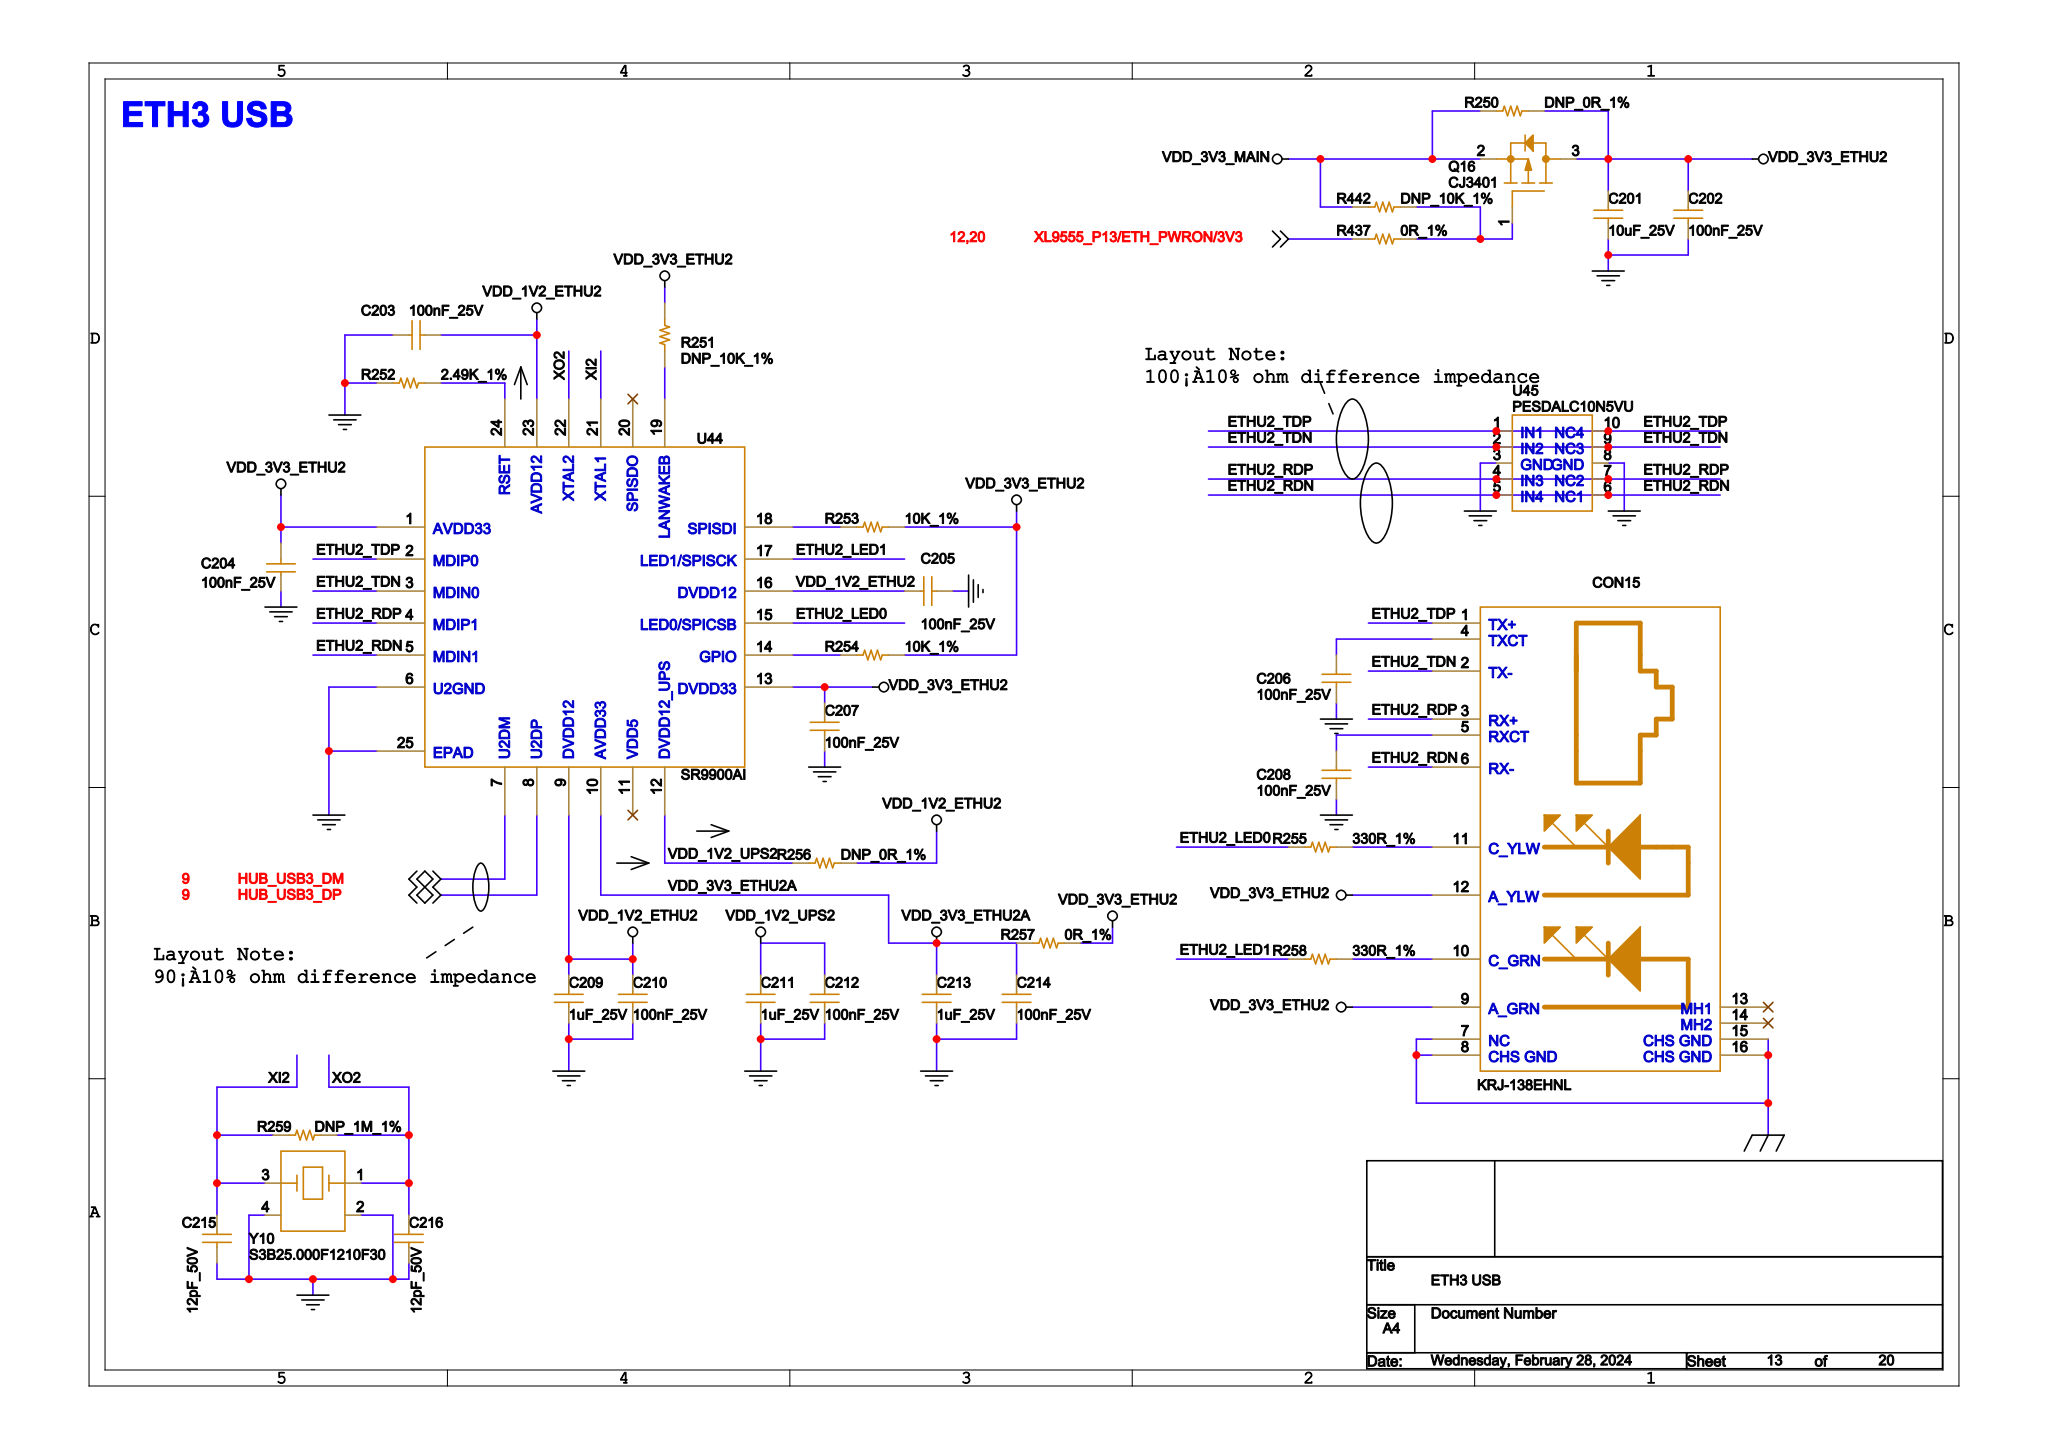Circuit board | Cadence Allegro | 1024 parts | 682 nets | one sheet of the schematic
Parts on this sheet (reference | value | footprint):
C201 | 10uF_25V | C0603
C202 | 100nF_25V | C0402
C203 | 100nF_25V | C0402
C204 | 100nF_25V | C0402
C205 | 100nF_25V | C0402
C206 | 100nF_25V | C0402
C207 | 100nF_25V | C0402
C208 | 100nF_25V | C0402
C209 | 1uF_25V | C0603
C210 | 100nF_25V | C0402
C211 | 1uF_25V | C0603
C212 | 100nF_25V | C0402
C213 | 1uF_25V | C0603
C214 | 100nF_25V | C0402
C215 | 12pF_50V | C0402
C216 | 12pF_50V | C0402
CON15 | KRJ-138EHNL | CON_YDS_13F-64GYD2PLXNL
Q16 | CJ3401 | SOT23-3
R250 | DNP_0R_1% | R0603
R251 | DNP_10K_1% | R0402
R252 | 2.49K_1% | R0603
R253 | 10K_1% | R0402
R254 | 10K_1% | R0402
R255 | 330R_1% | R0402
R256 | DNP_0R_1% | R0603
R257 | 0R_1% | R0603
R258 | 330R_1% | R0402
R259 | DNP_1M_1% | R0603
R437 | 0R_1% | R0402
R442 | DNP_10K_1% | R0402
U44 | SR9900AI | QFN24-4X4-0D5
U45 | PESDALC10N5VU | DFN-10-2510
Y10 | S3B25.000F1210F30 | SMD_3225
Nets of these parts (net: part-pin ...):
GND: C201-2 C202-2 C203-1 C204-1 C205-2 C206-2 C207-2 C208-2 C209-2 C210-2 C211-2 C212-2 C213-2 C214-2 C215-2 C216-2 R252-1 U45-3 U45-8 Y10-2 Y10-4 U44-6 U44-25
EGND: CON15-7 CON15-8 CON15-15 CON15-16
VDD_3V3_MAIN: Q16-2 R250-1 R442-1
XI2: C215-1 R259-2 Y10-3 U44-21
XO2: C216-1 R259-1 Y10-1 U44-22
VDD_3V3_ETHU2: C201-1 C202-1 C204-2 C207-1 CON15-9 CON15-12 Q16-3 R250-2 R251-2 R253-2 R254-2 R257-2 U44-1 U44-13
N21612959: CON15-10 R258-2
N21613044: CON15-11 R255-2
ETHU2_RDP: CON15-3 U45-4 U45-7 U44-4
ETHU2_RDN: CON15-6 U45-5 U45-6 U44-5
N21612403: C208-1 CON15-5
ETHU2_TDP: CON15-1 U45-1 U45-10 U44-2
ETHU2_TDN: CON15-2 U45-2 U45-9 U44-3
N21612986: C206-1 CON15-4
VDD_1V2_UPS2: C211-1 C212-1 R256-1 U44-12
VDD_1V2_ETHU2: C203-2 C205-1 C209-1 C210-1 R256-2 U44-9 U44-16 U44-23
VDD_3V3_ETHU2A: C213-1 C214-1 R257-1 U44-10
N21612772: R252-2 U44-24
ETHU2_LED0: R255-1 U44-15
ETHU2_LED1: R258-1 U44-17
N21612798: R254-1 U44-14
N21612604: R251-1 U44-19
N21612783: R253-1 U44-18
HUB_USB3_DM: U44-7
HUB_USB3_DP: U44-8
XL9555_P13/ETH_PWRON/3V3: R437-2
N22259098: Q16-1 R437-1 R442-2